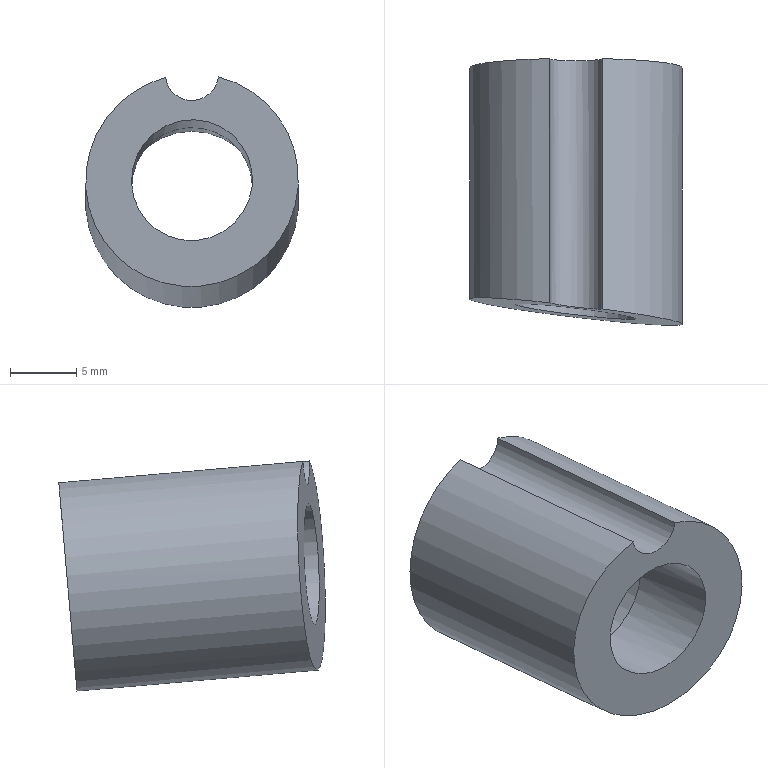Part | NX | features EKSD 16-20-7.100 2 | 1 solid | 7 faces | box 16 x 20.037 x 17.337 mm | volume 2113 mm3 | cylinder 4 | plane 3 | commonest cylinder face diameters 4 x1 9.1 x1 10.6 x1 16 x1
STEP:
#1=CARTESIAN_POINT('',(-696.404,-38.902,-29.923));
#2=VERTEX_POINT('',#1);
#3=CARTESIAN_POINT('',(-692.435,-38.902,-29.923));
#4=VERTEX_POINT('',#3);
#5=CARTESIAN_POINT('',(-694.42,-38.881,-29.674));
#6=DIRECTION('',(0.,-0.9962,0.08716));
#7=DIRECTION('',(0.,-0.08716,-0.9962));
#8=AXIS2_PLACEMENT_3D('',#5,#6,#7);
#9=CIRCLE('',#8,2.);
#10=EDGE_CURVE('',#2,#4,#9,.T.);
#11=ORIENTED_EDGE('',*,*,#10,.T.);
#12=CARTESIAN_POINT('',(-694.42,-39.578,-37.644));
#13=DIRECTION('',(0.,-0.9962,0.08716));
#14=DIRECTION('',(0.,-0.08716,-0.9962));
#15=AXIS2_PLACEMENT_3D('',#12,#13,#14);
#16=CIRCLE('',#15,8.);
#17=EDGE_CURVE('',#2,#4,#16,.T.);
#18=ORIENTED_EDGE('',*,*,#17,.F.);
#19=EDGE_LOOP('',(#11,#18));
#20=FACE_BOUND('',#19,.T.);
#21=CARTESIAN_POINT('',(-694.42,-39.116,-32.364));
#22=VERTEX_POINT('',#21);
#23=CARTESIAN_POINT('',(-694.42,-39.578,-37.644));
#24=DIRECTION('',(0.,0.9962,-0.08716));
#25=DIRECTION('',(0.,0.08716,0.9962));
#26=AXIS2_PLACEMENT_3D('',#23,#24,#25);
#27=CIRCLE('',#26,5.3);
#28=EDGE_CURVE('',#22,#22,#27,.T.);
#29=ORIENTED_EDGE('',*,*,#28,.F.);
#30=EDGE_LOOP('',(#29));
#31=FACE_BOUND('',#30,.T.);
#32=CARTESIAN_POINT('',(-694.42,-39.578,-37.644));
#33=DIRECTION('',(0.,0.9962,-0.08716));
#34=DIRECTION('',(0.,0.08716,0.9962));
#35=AXIS2_PLACEMENT_3D('',#32,#33,#34);
#36=PLANE('',#35);
#37=ADVANCED_FACE('',(#20,#31),#36,.T.);
#38=CARTESIAN_POINT('',(-692.435,-57.727,-28.276));
#39=VERTEX_POINT('',#38);
#40=CARTESIAN_POINT('',(-696.404,-57.259,-28.317));
#41=VERTEX_POINT('',#40);
#42=CARTESIAN_POINT('',(-694.42,-57.48,-28.047));
#43=DIRECTION('',(0.1175,0.9917,-0.05271));
#44=DIRECTION('',(-0.9536,0.09785,-0.2849));
#45=AXIS2_PLACEMENT_3D('',#42,#43,#44);
#46=ELLIPSE('',#45,2.015,2.);
#47=EDGE_CURVE('',#39,#41,#46,.T.);
#48=ORIENTED_EDGE('',*,*,#47,.T.);
#49=CARTESIAN_POINT('',(-694.42,-57.905,-36.04));
#50=DIRECTION('',(0.1175,0.9917,-0.05271));
#51=DIRECTION('',(-0.9536,0.09785,-0.2849));
#52=AXIS2_PLACEMENT_3D('',#49,#50,#51);
#53=ELLIPSE('',#52,8.061,8.);
#54=EDGE_CURVE('',#39,#41,#53,.T.);
#55=ORIENTED_EDGE('',*,*,#54,.F.);
#56=EDGE_LOOP('',(#48,#55));
#57=FACE_BOUND('',#56,.T.);
#58=CARTESIAN_POINT('',(-698.791,-57.456,-37.346));
#59=VERTEX_POINT('',#58);
#60=CARTESIAN_POINT('',(-694.42,-57.905,-36.04));
#61=DIRECTION('',(0.1175,0.9917,-0.05271));
#62=DIRECTION('',(-0.9536,0.09785,-0.2849));
#63=AXIS2_PLACEMENT_3D('',#60,#61,#62);
#64=ELLIPSE('',#63,4.584,4.55);
#65=EDGE_CURVE('',#59,#59,#64,.F.);
#66=ORIENTED_EDGE('',*,*,#65,.F.);
#67=EDGE_LOOP('',(#66));
#68=FACE_BOUND('',#67,.T.);
#69=CARTESIAN_POINT('',(-865.481,-35.468,4.737));
#70=DIRECTION('',(0.1175,0.9917,-0.05271));
#71=DIRECTION('',(0.05221,-0.05917,-0.9969));
#72=AXIS2_PLACEMENT_3D('',#69,#70,#71);
#73=PLANE('',#72);
#74=ADVANCED_FACE('',(#57,#68),#73,.F.);
#75=CARTESIAN_POINT('',(-692.435,-48.864,-29.052));
#76=DIRECTION('',(0.,0.9962,-0.08716));
#77=VECTOR('',#76,1000.);
#78=LINE('',#75,#77);
#79=EDGE_CURVE('',#39,#4,#78,.T.);
#80=ORIENTED_EDGE('',*,*,#79,.F.);
#81=ORIENTED_EDGE('',*,*,#54,.T.);
#82=CARTESIAN_POINT('',(-696.404,-48.864,-29.052));
#83=DIRECTION('',(0.,0.9962,-0.08716));
#84=VECTOR('',#83,1000.);
#85=LINE('',#82,#84);
#86=EDGE_CURVE('',#2,#41,#85,.F.);
#87=ORIENTED_EDGE('',*,*,#86,.F.);
#88=ORIENTED_EDGE('',*,*,#17,.T.);
#89=EDGE_LOOP('',(#80,#81,#87,#88));
#90=FACE_BOUND('',#89,.T.);
#91=CARTESIAN_POINT('',(-694.42,-59.502,-35.901));
#92=DIRECTION('',(0.,0.9962,-0.08716));
#93=DIRECTION('',(0.,0.08716,0.9962));
#94=AXIS2_PLACEMENT_3D('',#91,#92,#93);
#95=CYLINDRICAL_SURFACE('',#94,8.);
#96=ADVANCED_FACE('',(#90),#95,.T.);
#97=CARTESIAN_POINT('',(-694.42,-51.929,-41.131));
#98=VERTEX_POINT('',#97);
#99=CARTESIAN_POINT('',(-694.42,-51.532,-36.598));
#100=DIRECTION('',(0.,-0.9962,0.08716));
#101=DIRECTION('',(0.,-0.08716,-0.9962));
#102=AXIS2_PLACEMENT_3D('',#99,#100,#101);
#103=CIRCLE('',#102,4.55);
#104=EDGE_CURVE('',#98,#98,#103,.F.);
#105=ORIENTED_EDGE('',*,*,#104,.T.);
#106=EDGE_LOOP('',(#105));
#107=FACE_BOUND('',#106,.T.);
#108=ORIENTED_EDGE('',*,*,#65,.T.);
#109=EDGE_LOOP('',(#108));
#110=FACE_BOUND('',#109,.T.);
#111=CARTESIAN_POINT('',(-694.42,-60.498,-35.813));
#112=DIRECTION('',(0.,0.9962,-0.08716));
#113=DIRECTION('',(0.,0.08716,0.9962));
#114=AXIS2_PLACEMENT_3D('',#111,#112,#113);
#115=CYLINDRICAL_SURFACE('',#114,4.55);
#116=ADVANCED_FACE('',(#107,#110),#115,.F.);
#117=CARTESIAN_POINT('',(-694.42,-51.07,-31.318));
#118=VERTEX_POINT('',#117);
#119=CARTESIAN_POINT('',(-694.42,-51.532,-36.598));
#120=DIRECTION('',(0.,0.9962,-0.08716));
#121=DIRECTION('',(0.,0.08716,0.9962));
#122=AXIS2_PLACEMENT_3D('',#119,#120,#121);
#123=CIRCLE('',#122,5.3);
#124=EDGE_CURVE('',#118,#118,#123,.T.);
#125=ORIENTED_EDGE('',*,*,#124,.T.);
#126=EDGE_LOOP('',(#125));
#127=FACE_BOUND('',#126,.T.);
#128=ORIENTED_EDGE('',*,*,#104,.F.);
#129=EDGE_LOOP('',(#128));
#130=FACE_BOUND('',#129,.T.);
#131=CARTESIAN_POINT('',(-694.42,-51.532,-36.598));
#132=DIRECTION('',(0.,-0.9962,0.08716));
#133=DIRECTION('',(0.,-0.08716,-0.9962));
#134=AXIS2_PLACEMENT_3D('',#131,#132,#133);
#135=PLANE('',#134);
#136=ADVANCED_FACE('',(#127,#130),#135,.F.);
#137=ORIENTED_EDGE('',*,*,#28,.T.);
#138=EDGE_LOOP('',(#137));
#139=FACE_BOUND('',#138,.T.);
#140=ORIENTED_EDGE('',*,*,#124,.F.);
#141=EDGE_LOOP('',(#140));
#142=FACE_BOUND('',#141,.T.);
#143=CARTESIAN_POINT('',(-694.42,-51.532,-36.598));
#144=DIRECTION('',(0.,0.9962,-0.08716));
#145=DIRECTION('',(0.,0.08716,0.9962));
#146=AXIS2_PLACEMENT_3D('',#143,#144,#145);
#147=CYLINDRICAL_SURFACE('',#146,5.3);
#148=ADVANCED_FACE('',(#139,#142),#147,.F.);
#149=ORIENTED_EDGE('',*,*,#79,.T.);
#150=ORIENTED_EDGE('',*,*,#10,.F.);
#151=ORIENTED_EDGE('',*,*,#86,.T.);
#152=ORIENTED_EDGE('',*,*,#47,.F.);
#153=EDGE_LOOP('',(#149,#150,#151,#152));
#154=FACE_BOUND('',#153,.T.);
#155=CARTESIAN_POINT('',(-694.42,-58.804,-27.931));
#156=DIRECTION('',(0.,0.9962,-0.08716));
#157=DIRECTION('',(0.,0.08716,0.9962));
#158=AXIS2_PLACEMENT_3D('',#155,#156,#157);
#159=CYLINDRICAL_SURFACE('',#158,2.);
#160=ADVANCED_FACE('',(#154),#159,.F.);
#161=CLOSED_SHELL('',(#37,#74,#96,#116,#136,#148,#160));
#162=MANIFOLD_SOLID_BREP('',#161);
#163=(LENGTH_UNIT()NAMED_UNIT(*)SI_UNIT(.MILLI.,.METRE.));
#164=UNCERTAINTY_MEASURE_WITH_UNIT(LENGTH_MEASURE(0.00001),#163,'','');
#165=(NAMED_UNIT(*)PLANE_ANGLE_UNIT()SI_UNIT($,.RADIAN.));
#166=(NAMED_UNIT(*)SI_UNIT($,.STERADIAN.)SOLID_ANGLE_UNIT());
#167=(GEOMETRIC_REPRESENTATION_CONTEXT(3)GLOBAL_UNCERTAINTY_ASSIGNED_CONTEXT((#164))GLOBAL_UNIT_ASSIGNED_CONTEXT((#163,#165,#166))REPRESENTATION_CONTEXT('',''));
#168=ADVANCED_BREP_SHAPE_REPRESENTATION('',(#162),#167);